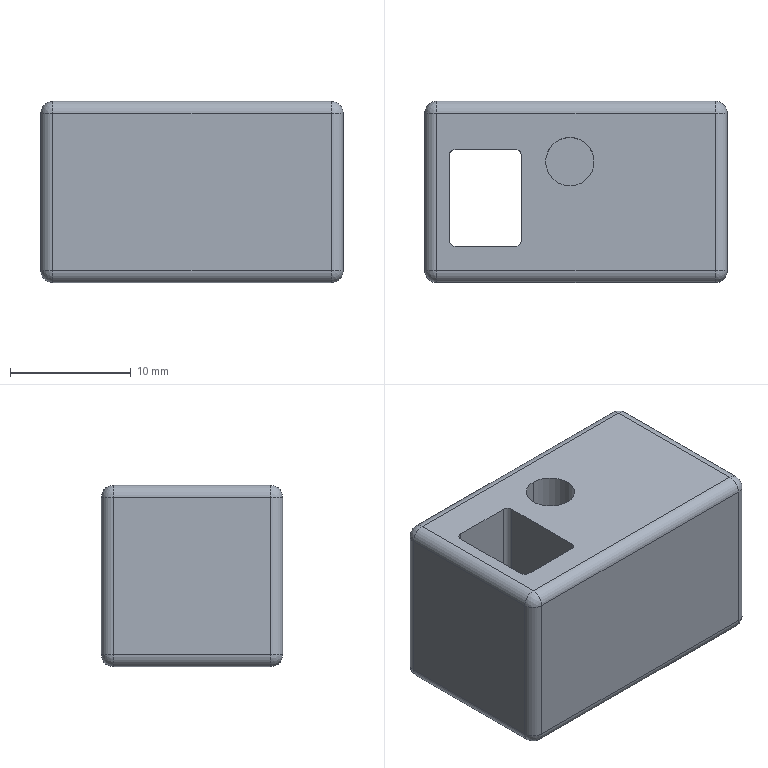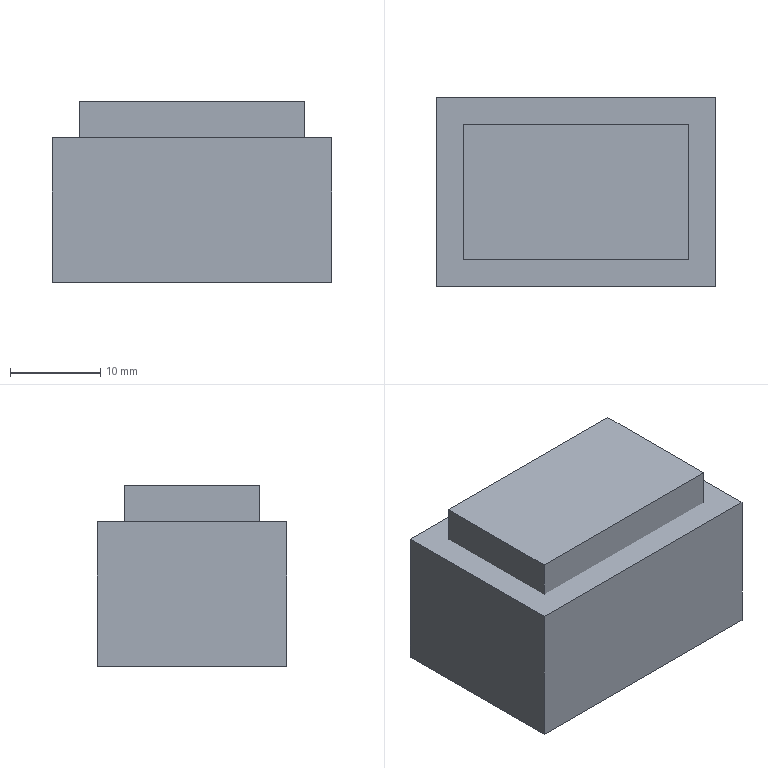CAM job | NX | 3-axis milling | part box 25 x 15 x 15 mm | stock box 31 x 21 x 20 mm
Tools:
number,name,description,diameter,corner_radius,flute_length,length,flutes
1,D63,Milling Tool-5 Parameters,63.0,0.0,50.0,75.0,2
9,D10,Milling Tool-5 Parameters,10.0,0.0,50.0,75.0,2
4,D4,Milling Tool-5 Parameters,4.0,0.0,50.0,75.0,2
3,D3,Milling Tool-5 Parameters,3.0,0.0,50.0,75.0,2
10,D10JING,Milling Tool-5 Parameters,10.0,0.0,50.0,75.0,2
8,D6R0.5,Milling Tool-5 Parameters,6.0,0.5,50.0,75.0,2
2,D4A45,Milling Tool-5 Parameters,4.0,0.0,2.0,2.0,2
12,D2,Milling Tool-5 Parameters,2.0,0.0,50.0,75.0,2
Operations:
program,operation,operation_type,tool,method,geometry_group,spindle_rpm,surface_speed,feed_per_tooth,feed_cut,feed_plunge,cut_length_mm,path_length_mm,cut_time_min,machine_time_min
1虎钳,FLOOR_WALL,VolumeBased25DMillingOperation,D63,METHOD,A,6500.0,1286.0,0.0962,1250.0,100.0,106.0,160.0,0.0848,0.0902
1虎钳,ZLEVEL_PROFILE,ZLevelMilling,D10,METHOD,A,9500.0,298.0,0.1579,3000.0,1000.0,1761.543,1833.543,0.619,0.6262
1虎钳,ZLEVEL_PROFILE_COPY_COPY,ZLevelMilling,D10JING,METHOD,A,9500.0,119.0,0.0632,1200.0,1000.0,118.063,205.063,0.0991,0.1078
1虎钳,ZLEVEL_PROFILE_COPY_1,ZLevelMilling,D6R0.5,METHOD,A,9500.0,179.0,0.1579,3000.0,1000.0,2176.432,2234.944,0.7276,0.7334
1虎钳,ZLEVEL_PROFILE_COPY,ZLevelMilling,D4,METHOD,A,9500.0,119.0,0.0789,1500.0,1000.0,503.024,575.024,0.3474,0.3546
1虎钳,ZLEVEL_PROFILE_COPY_COPY_1,ZLevelMilling,D3,METHOD,A,9500.0,119.0,0.0789,1500.0,1000.0,51.279,115.279,0.0398,0.0462
1虎钳,CAVITY_MILL_COPY_COPY,CavityMilling,D2,METHOD,A,9500.0,44.0,0.0579,1100.0,1000.0,1660.582,2841.98,1.543,1.661
1虎钳,ZLEVEL_PROFILE_1_COPY_1_COPY,ZLevelMilling,D4A45,METHOD,A,9500.0,179.0,0.0526,1000.0,100.0,35.702,163.908,0.0357,0.0485
1虎钳,刀补4,CylinderMilling,D3,METHOD,A,9500.0,119.0,0.0526,1000.0,100.0,25.678,90.178,0.0257,0.0321
2,FLOOR_WALL_COPY,VolumeBased25DMillingOperation,D63,METHOD,B,6500.0,1286.0,0.0962,1250.0,100.0,500.0,1126.001,0.4,0.4626
2,ZLEVEL_PROFILE_COPY_1_COPY,ZLevelMilling,D6R0.5,METHOD,B,9500.0,179.0,0.1579,3000.0,1000.0,2176.432,2234.944,0.7276,0.7334
2,ZLEVEL_PROFILE_1_COPY_1_COPY_COPY,ZLevelMilling,D4A45,METHOD,B,9500.0,179.0,0.0526,1000.0,100.0,24.983,84.984,0.025,0.031